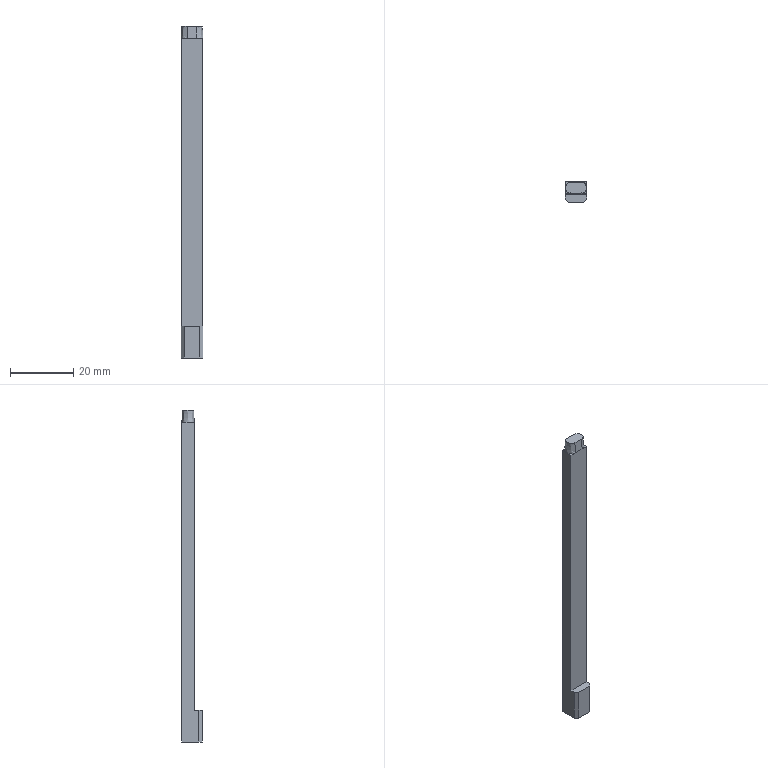Part | Creo | 1 solid | 137 faces | box 6.926 x 6.418 x 105.073 mm | volume 2991 mm3 | other 79 | plane 55 | spline 2 | cylinder 1 | commonest cylinder face diameters 8.215 x1